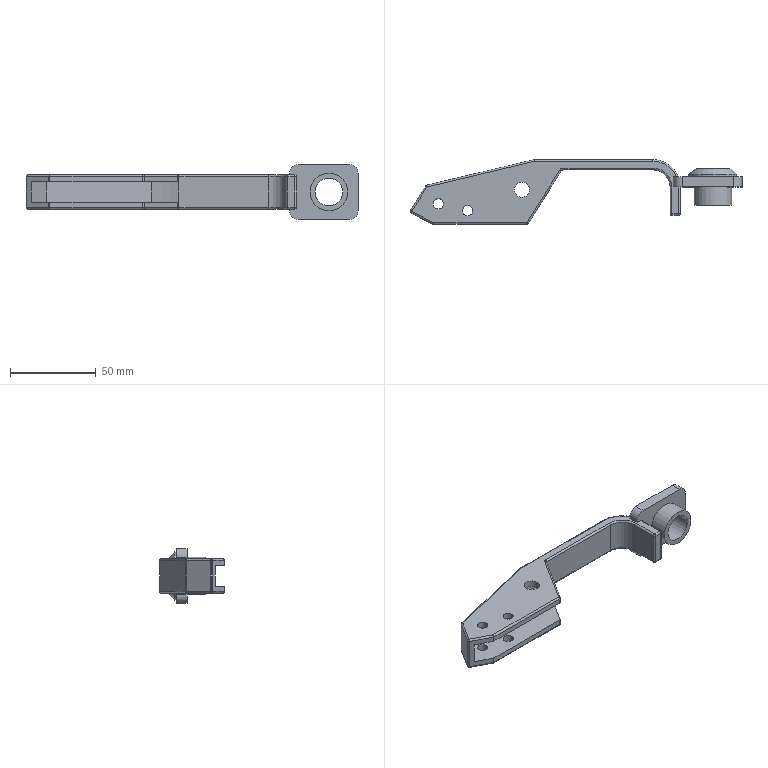Part | STEP file | 1 solid | 106 faces | box 193.54 x 37.8 x 32 mm | volume 42098 mm3 | cylinder 57 | plane 27 | sphere 14 | torus 6 | cone 2 | commonest cylinder face diameters 2 x32 6 x8 9 x4 10 x4 16 x2 22 x2